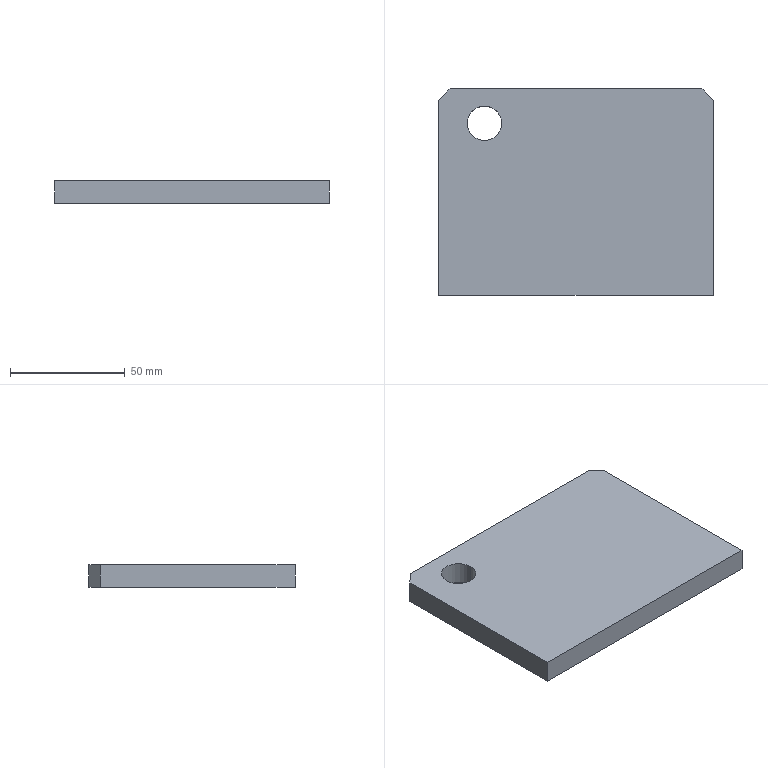Part | SolidWorks | features Chamfer 1, Extrusion 1, ICE 1 | 1 solid | 10 faces | box 120 x 90 x 10 mm | volume 105983 mm3 | plane 8 | cylinder 2 | commonest cylinder face diameters 15 x2
STEP:
#1=CARTESIAN_POINT('',(-47.5,30.,0.));
#2=VERTEX_POINT('',#1);
#3=CARTESIAN_POINT('',(-32.5,30.,0.));
#4=VERTEX_POINT('',#3);
#5=CARTESIAN_POINT('',(-40.,30.,0.));
#6=DIRECTION('',(0.,0.,1.));
#7=DIRECTION('',(1.,0.,0.));
#8=AXIS2_PLACEMENT_3D('',#5,#6,#7);
#9=CIRCLE('',#8,7.5);
#10=EDGE_CURVE('',#2,#4,#9,.T.);
#11=ORIENTED_EDGE('',*,*,#10,.F.);
#12=CARTESIAN_POINT('',(-47.5,30.,10.));
#13=VERTEX_POINT('',#12);
#14=CARTESIAN_POINT('',(-47.5,30.,0.));
#15=DIRECTION('',(0.,0.,1.));
#16=VECTOR('',#15,1000.);
#17=LINE('',#14,#16);
#18=EDGE_CURVE('',#2,#13,#17,.T.);
#19=ORIENTED_EDGE('',*,*,#18,.T.);
#20=CARTESIAN_POINT('',(-32.5,30.,10.));
#21=VERTEX_POINT('',#20);
#22=CARTESIAN_POINT('',(-40.,30.,10.));
#23=DIRECTION('',(0.,0.,1.));
#24=DIRECTION('',(1.,0.,0.));
#25=AXIS2_PLACEMENT_3D('',#22,#23,#24);
#26=CIRCLE('',#25,7.5);
#27=EDGE_CURVE('',#13,#21,#26,.T.);
#28=ORIENTED_EDGE('',*,*,#27,.T.);
#29=CARTESIAN_POINT('',(-32.5,30.,0.));
#30=DIRECTION('',(0.,0.,1.));
#31=VECTOR('',#30,1000.);
#32=LINE('',#29,#31);
#33=EDGE_CURVE('',#4,#21,#32,.T.);
#34=ORIENTED_EDGE('',*,*,#33,.F.);
#35=EDGE_LOOP('',(#11,#19,#28,#34));
#36=FACE_OUTER_BOUND('',#35,.T.);
#37=CARTESIAN_POINT('',(-40.,30.,0.));
#38=DIRECTION('',(0.,0.,1.));
#39=DIRECTION('',(1.,0.,0.));
#40=AXIS2_PLACEMENT_3D('',#37,#38,#39);
#41=CYLINDRICAL_SURFACE('',#40,7.5);
#42=ADVANCED_FACE('',(#36),#41,.F.);
#43=CARTESIAN_POINT('',(-60.,40.,10.));
#44=VERTEX_POINT('',#43);
#45=CARTESIAN_POINT('',(-60.,-45.,10.));
#46=VERTEX_POINT('',#45);
#47=CARTESIAN_POINT('',(-60.,45.,10.));
#48=DIRECTION('',(0.,-1.,0.));
#49=VECTOR('',#48,1000.);
#50=LINE('',#47,#49);
#51=EDGE_CURVE('',#44,#46,#50,.T.);
#52=ORIENTED_EDGE('',*,*,#51,.F.);
#53=CARTESIAN_POINT('',(-60.,40.,0.));
#54=VERTEX_POINT('',#53);
#55=CARTESIAN_POINT('',(-60.,40.,10.));
#56=DIRECTION('',(0.,0.,-1.));
#57=VECTOR('',#56,1000.);
#58=LINE('',#55,#57);
#59=EDGE_CURVE('',#44,#54,#58,.T.);
#60=ORIENTED_EDGE('',*,*,#59,.T.);
#61=CARTESIAN_POINT('',(-60.,-45.,0.));
#62=VERTEX_POINT('',#61);
#63=CARTESIAN_POINT('',(-60.,45.,0.));
#64=DIRECTION('',(0.,-1.,0.));
#65=VECTOR('',#64,1000.);
#66=LINE('',#63,#65);
#67=EDGE_CURVE('',#54,#62,#66,.T.);
#68=ORIENTED_EDGE('',*,*,#67,.T.);
#69=CARTESIAN_POINT('',(-60.,-45.,10.));
#70=DIRECTION('',(0.,0.,-1.));
#71=VECTOR('',#70,1000.);
#72=LINE('',#69,#71);
#73=EDGE_CURVE('',#46,#62,#72,.T.);
#74=ORIENTED_EDGE('',*,*,#73,.F.);
#75=EDGE_LOOP('',(#52,#60,#68,#74));
#76=FACE_OUTER_BOUND('',#75,.T.);
#77=CARTESIAN_POINT('',(-60.,45.,10.));
#78=DIRECTION('',(1.,0.,0.));
#79=DIRECTION('',(0.,1.,0.));
#80=AXIS2_PLACEMENT_3D('',#77,#78,#79);
#81=PLANE('',#80);
#82=ADVANCED_FACE('',(#76),#81,.F.);
#83=CARTESIAN_POINT('',(60.,-45.,0.));
#84=VERTEX_POINT('',#83);
#85=CARTESIAN_POINT('',(60.,-45.,0.));
#86=DIRECTION('',(1.,0.,0.));
#87=VECTOR('',#86,1000.);
#88=LINE('',#85,#87);
#89=EDGE_CURVE('',#62,#84,#88,.T.);
#90=ORIENTED_EDGE('',*,*,#89,.T.);
#91=CARTESIAN_POINT('',(60.,-45.,10.));
#92=VERTEX_POINT('',#91);
#93=CARTESIAN_POINT('',(60.,-45.,10.));
#94=DIRECTION('',(0.,0.,-1.));
#95=VECTOR('',#94,1000.);
#96=LINE('',#93,#95);
#97=EDGE_CURVE('',#92,#84,#96,.T.);
#98=ORIENTED_EDGE('',*,*,#97,.F.);
#99=CARTESIAN_POINT('',(60.,-45.,10.));
#100=DIRECTION('',(1.,0.,0.));
#101=VECTOR('',#100,1000.);
#102=LINE('',#99,#101);
#103=EDGE_CURVE('',#46,#92,#102,.T.);
#104=ORIENTED_EDGE('',*,*,#103,.F.);
#105=ORIENTED_EDGE('',*,*,#73,.T.);
#106=EDGE_LOOP('',(#90,#98,#104,#105));
#107=FACE_OUTER_BOUND('',#106,.T.);
#108=CARTESIAN_POINT('',(60.,-45.,10.));
#109=DIRECTION('',(0.,1.,0.));
#110=DIRECTION('',(-1.,0.,0.));
#111=AXIS2_PLACEMENT_3D('',#108,#109,#110);
#112=PLANE('',#111);
#113=ADVANCED_FACE('',(#107),#112,.F.);
#114=CARTESIAN_POINT('',(60.,40.,0.));
#115=VERTEX_POINT('',#114);
#116=CARTESIAN_POINT('',(60.,45.,0.));
#117=DIRECTION('',(0.,1.,0.));
#118=VECTOR('',#117,1000.);
#119=LINE('',#116,#118);
#120=EDGE_CURVE('',#84,#115,#119,.T.);
#121=ORIENTED_EDGE('',*,*,#120,.T.);
#122=CARTESIAN_POINT('',(60.,40.,10.));
#123=VERTEX_POINT('',#122);
#124=CARTESIAN_POINT('',(60.,40.,10.));
#125=DIRECTION('',(0.,0.,1.));
#126=VECTOR('',#125,1000.);
#127=LINE('',#124,#126);
#128=EDGE_CURVE('',#115,#123,#127,.T.);
#129=ORIENTED_EDGE('',*,*,#128,.T.);
#130=CARTESIAN_POINT('',(60.,45.,10.));
#131=DIRECTION('',(0.,1.,0.));
#132=VECTOR('',#131,1000.);
#133=LINE('',#130,#132);
#134=EDGE_CURVE('',#92,#123,#133,.T.);
#135=ORIENTED_EDGE('',*,*,#134,.F.);
#136=ORIENTED_EDGE('',*,*,#97,.T.);
#137=EDGE_LOOP('',(#121,#129,#135,#136));
#138=FACE_OUTER_BOUND('',#137,.T.);
#139=CARTESIAN_POINT('',(60.,45.,10.));
#140=DIRECTION('',(-1.,0.,0.));
#141=DIRECTION('',(0.,-1.,0.));
#142=AXIS2_PLACEMENT_3D('',#139,#140,#141);
#143=PLANE('',#142);
#144=ADVANCED_FACE('',(#138),#143,.F.);
#145=CARTESIAN_POINT('',(55.,45.,10.));
#146=VERTEX_POINT('',#145);
#147=CARTESIAN_POINT('',(-55.,45.,10.));
#148=VERTEX_POINT('',#147);
#149=CARTESIAN_POINT('',(60.,45.,10.));
#150=DIRECTION('',(-1.,0.,0.));
#151=VECTOR('',#150,1000.);
#152=LINE('',#149,#151);
#153=EDGE_CURVE('',#146,#148,#152,.T.);
#154=ORIENTED_EDGE('',*,*,#153,.F.);
#155=CARTESIAN_POINT('',(55.,45.,0.));
#156=VERTEX_POINT('',#155);
#157=CARTESIAN_POINT('',(55.,45.,10.));
#158=DIRECTION('',(0.,0.,-1.));
#159=VECTOR('',#158,1000.);
#160=LINE('',#157,#159);
#161=EDGE_CURVE('',#146,#156,#160,.T.);
#162=ORIENTED_EDGE('',*,*,#161,.T.);
#163=CARTESIAN_POINT('',(-55.,45.,0.));
#164=VERTEX_POINT('',#163);
#165=CARTESIAN_POINT('',(60.,45.,0.));
#166=DIRECTION('',(-1.,0.,0.));
#167=VECTOR('',#166,1000.);
#168=LINE('',#165,#167);
#169=EDGE_CURVE('',#156,#164,#168,.T.);
#170=ORIENTED_EDGE('',*,*,#169,.T.);
#171=CARTESIAN_POINT('',(-55.,45.,10.));
#172=DIRECTION('',(0.,0.,1.));
#173=VECTOR('',#172,1000.);
#174=LINE('',#171,#173);
#175=EDGE_CURVE('',#164,#148,#174,.T.);
#176=ORIENTED_EDGE('',*,*,#175,.T.);
#177=EDGE_LOOP('',(#154,#162,#170,#176));
#178=FACE_OUTER_BOUND('',#177,.T.);
#179=CARTESIAN_POINT('',(60.,45.,10.));
#180=DIRECTION('',(0.,-1.,0.));
#181=DIRECTION('',(1.,0.,0.));
#182=AXIS2_PLACEMENT_3D('',#179,#180,#181);
#183=PLANE('',#182);
#184=ADVANCED_FACE('',(#178),#183,.F.);
#185=CARTESIAN_POINT('',(-40.,30.,10.));
#186=DIRECTION('',(0.,0.,1.));
#187=DIRECTION('',(1.,0.,0.));
#188=AXIS2_PLACEMENT_3D('',#185,#186,#187);
#189=CIRCLE('',#188,7.5);
#190=EDGE_CURVE('',#21,#13,#189,.T.);
#191=ORIENTED_EDGE('',*,*,#190,.F.);
#192=ORIENTED_EDGE('',*,*,#27,.F.);
#193=EDGE_LOOP('',(#191,#192));
#194=FACE_BOUND('',#193,.T.);
#195=ORIENTED_EDGE('',*,*,#134,.T.);
#196=CARTESIAN_POINT('',(55.,45.,10.));
#197=DIRECTION('',(-0.7071,0.7071,0.));
#198=VECTOR('',#197,1000.);
#199=LINE('',#196,#198);
#200=EDGE_CURVE('',#123,#146,#199,.T.);
#201=ORIENTED_EDGE('',*,*,#200,.T.);
#202=ORIENTED_EDGE('',*,*,#153,.T.);
#203=CARTESIAN_POINT('',(-60.,40.,10.));
#204=DIRECTION('',(-0.7071,-0.7071,0.));
#205=VECTOR('',#204,1000.);
#206=LINE('',#203,#205);
#207=EDGE_CURVE('',#148,#44,#206,.T.);
#208=ORIENTED_EDGE('',*,*,#207,.T.);
#209=ORIENTED_EDGE('',*,*,#51,.T.);
#210=ORIENTED_EDGE('',*,*,#103,.T.);
#211=EDGE_LOOP('',(#195,#201,#202,#208,#209,#210));
#212=FACE_OUTER_BOUND('',#211,.T.);
#213=CARTESIAN_POINT('',(0.,0.,10.));
#214=DIRECTION('',(0.,0.,-1.));
#215=DIRECTION('',(-1.,0.,0.));
#216=AXIS2_PLACEMENT_3D('',#213,#214,#215);
#217=PLANE('',#216);
#218=ADVANCED_FACE('',(#194,#212),#217,.F.);
#219=CARTESIAN_POINT('',(-40.,30.,0.));
#220=DIRECTION('',(0.,0.,1.));
#221=DIRECTION('',(1.,0.,0.));
#222=AXIS2_PLACEMENT_3D('',#219,#220,#221);
#223=CIRCLE('',#222,7.5);
#224=EDGE_CURVE('',#4,#2,#223,.T.);
#225=ORIENTED_EDGE('',*,*,#224,.T.);
#226=ORIENTED_EDGE('',*,*,#10,.T.);
#227=EDGE_LOOP('',(#225,#226));
#228=FACE_BOUND('',#227,.T.);
#229=ORIENTED_EDGE('',*,*,#169,.F.);
#230=CARTESIAN_POINT('',(50.,50.,0.));
#231=DIRECTION('',(0.7071,-0.7071,0.));
#232=VECTOR('',#231,1000.);
#233=LINE('',#230,#232);
#234=EDGE_CURVE('',#156,#115,#233,.T.);
#235=ORIENTED_EDGE('',*,*,#234,.T.);
#236=ORIENTED_EDGE('',*,*,#120,.F.);
#237=ORIENTED_EDGE('',*,*,#89,.F.);
#238=ORIENTED_EDGE('',*,*,#67,.F.);
#239=CARTESIAN_POINT('',(-50.,50.,0.));
#240=DIRECTION('',(0.7071,0.7071,0.));
#241=VECTOR('',#240,1000.);
#242=LINE('',#239,#241);
#243=EDGE_CURVE('',#54,#164,#242,.T.);
#244=ORIENTED_EDGE('',*,*,#243,.T.);
#245=EDGE_LOOP('',(#229,#235,#236,#237,#238,#244));
#246=FACE_OUTER_BOUND('',#245,.T.);
#247=CARTESIAN_POINT('',(0.,0.,0.));
#248=DIRECTION('',(0.,0.,-1.));
#249=DIRECTION('',(-1.,0.,0.));
#250=AXIS2_PLACEMENT_3D('',#247,#248,#249);
#251=PLANE('',#250);
#252=ADVANCED_FACE('',(#228,#246),#251,.T.);
#253=ORIENTED_EDGE('',*,*,#18,.F.);
#254=ORIENTED_EDGE('',*,*,#224,.F.);
#255=ORIENTED_EDGE('',*,*,#33,.T.);
#256=ORIENTED_EDGE('',*,*,#190,.T.);
#257=EDGE_LOOP('',(#253,#254,#255,#256));
#258=FACE_OUTER_BOUND('',#257,.T.);
#259=CARTESIAN_POINT('',(-40.,30.,0.));
#260=DIRECTION('',(0.,0.,1.));
#261=DIRECTION('',(1.,0.,0.));
#262=AXIS2_PLACEMENT_3D('',#259,#260,#261);
#263=CYLINDRICAL_SURFACE('',#262,7.5);
#264=ADVANCED_FACE('',(#258),#263,.F.);
#265=ORIENTED_EDGE('',*,*,#200,.F.);
#266=ORIENTED_EDGE('',*,*,#128,.F.);
#267=ORIENTED_EDGE('',*,*,#234,.F.);
#268=ORIENTED_EDGE('',*,*,#161,.F.);
#269=EDGE_LOOP('',(#265,#266,#267,#268));
#270=FACE_OUTER_BOUND('',#269,.T.);
#271=CARTESIAN_POINT('',(55.,45.,10.));
#272=DIRECTION('',(-0.7071,-0.7071,0.));
#273=DIRECTION('',(0.,0.,-1.));
#274=AXIS2_PLACEMENT_3D('',#271,#272,#273);
#275=PLANE('',#274);
#276=ADVANCED_FACE('',(#270),#275,.F.);
#277=ORIENTED_EDGE('',*,*,#207,.F.);
#278=ORIENTED_EDGE('',*,*,#175,.F.);
#279=ORIENTED_EDGE('',*,*,#243,.F.);
#280=ORIENTED_EDGE('',*,*,#59,.F.);
#281=EDGE_LOOP('',(#277,#278,#279,#280));
#282=FACE_OUTER_BOUND('',#281,.T.);
#283=CARTESIAN_POINT('',(-60.,40.,10.));
#284=DIRECTION('',(0.7071,-0.7071,0.));
#285=DIRECTION('',(0.,0.,-1.));
#286=AXIS2_PLACEMENT_3D('',#283,#284,#285);
#287=PLANE('',#286);
#288=ADVANCED_FACE('',(#282),#287,.F.);
#289=CLOSED_SHELL('',(#42,#82,#113,#144,#184,#218,#252,#264,#276,#288));
#290=MANIFOLD_SOLID_BREP('',#289);
#291=CARTESIAN_POINT('',(0.,0.,0.));
#292=DIRECTION('',(0.,0.,1.));
#293=DIRECTION('',(1.,0.,0.));
#294=AXIS2_PLACEMENT_3D('',#291,#292,#293);
#295=(LENGTH_UNIT()NAMED_UNIT(*)SI_UNIT(.MILLI.,.METRE.));
#296=UNCERTAINTY_MEASURE_WITH_UNIT(LENGTH_MEASURE(0.00001),#295,'','');
#297=(NAMED_UNIT(*)PLANE_ANGLE_UNIT()SI_UNIT($,.RADIAN.));
#298=(NAMED_UNIT(*)SI_UNIT($,.STERADIAN.)SOLID_ANGLE_UNIT());
#299=(GEOMETRIC_REPRESENTATION_CONTEXT(3)GLOBAL_UNCERTAINTY_ASSIGNED_CONTEXT((#296))GLOBAL_UNIT_ASSIGNED_CONTEXT((#295,#297,#298))REPRESENTATION_CONTEXT('',''));
#300=ADVANCED_BREP_SHAPE_REPRESENTATION('',(#290,#294),#299);